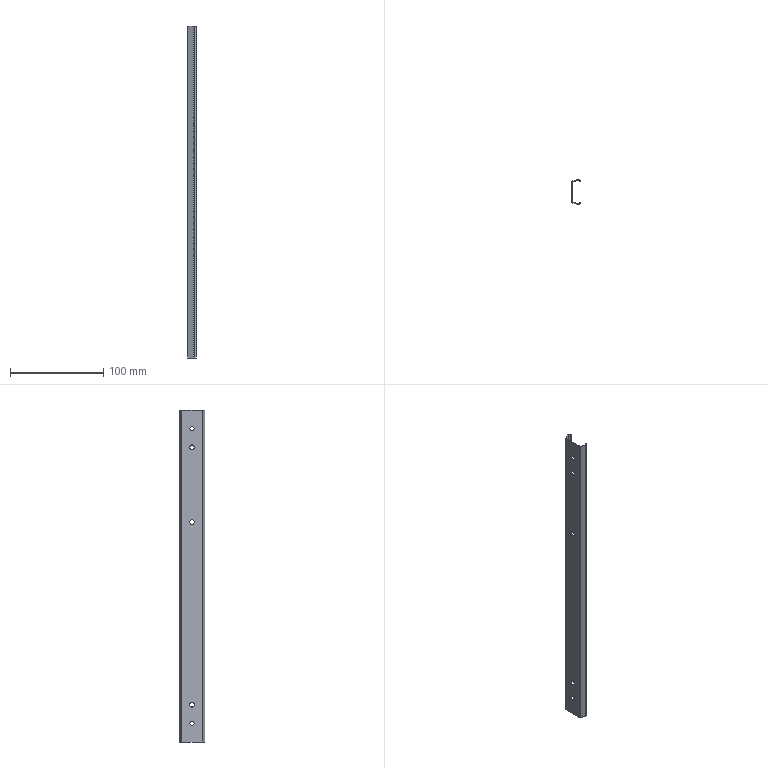Part | SolidWorks | features BaseBody 1, RefAxis 1 | 1 solid | 37 faces | box 9 x 27 x 355.6 mm | volume 7594 mm3 | plane 20 | cylinder 17 | commonest cylinder face diameters 4.5 x13 3.7 x2 3.8 x2
STEP:
#1=CARTESIAN_POINT('',(-2.55,11.15,333.35));
#2=VERTEX_POINT('',#1);
#3=CARTESIAN_POINT('',(-2.55,11.15,337.85));
#4=VERTEX_POINT('',#3);
#5=CARTESIAN_POINT('',(-2.55,11.15,335.6));
#6=DIRECTION('',(-1.,0.,0.));
#7=DIRECTION('',(0.,0.,1.));
#8=AXIS2_PLACEMENT_3D('',#5,#6,#7);
#9=CIRCLE('',#8,2.25);
#10=EDGE_CURVE('',#2,#4,#9,.T.);
#11=ORIENTED_EDGE('',*,*,#10,.F.);
#12=CARTESIAN_POINT('',(-3.05,11.15,333.35));
#13=VERTEX_POINT('',#12);
#14=CARTESIAN_POINT('',(-3.05,11.15,333.35));
#15=DIRECTION('',(-1.,0.,0.));
#16=VECTOR('',#15,1000.);
#17=LINE('',#14,#16);
#18=EDGE_CURVE('',#2,#13,#17,.T.);
#19=ORIENTED_EDGE('',*,*,#18,.T.);
#20=CARTESIAN_POINT('',(-3.05,11.15,337.85));
#21=VERTEX_POINT('',#20);
#22=CARTESIAN_POINT('',(-3.05,11.15,335.6));
#23=DIRECTION('',(1.,0.,0.));
#24=DIRECTION('',(0.,0.,1.));
#25=AXIS2_PLACEMENT_3D('',#22,#23,#24);
#26=CIRCLE('',#25,2.25);
#27=EDGE_CURVE('',#21,#13,#26,.T.);
#28=ORIENTED_EDGE('',*,*,#27,.F.);
#29=CARTESIAN_POINT('',(-3.05,11.15,337.85));
#30=DIRECTION('',(-1.,0.,0.));
#31=VECTOR('',#30,1000.);
#32=LINE('',#29,#31);
#33=EDGE_CURVE('',#4,#21,#32,.T.);
#34=ORIENTED_EDGE('',*,*,#33,.F.);
#35=EDGE_LOOP('',(#11,#19,#28,#34));
#36=FACE_OUTER_BOUND('',#35,.T.);
#37=CARTESIAN_POINT('',(-3.05,11.15,335.6));
#38=DIRECTION('',(-1.,0.,0.));
#39=DIRECTION('',(0.,0.,1.));
#40=AXIS2_PLACEMENT_3D('',#37,#38,#39);
#41=CYLINDRICAL_SURFACE('',#40,2.25);
#42=ADVANCED_FACE('',(#36),#41,.F.);
#43=CARTESIAN_POINT('',(-2.55,11.15,17.75));
#44=VERTEX_POINT('',#43);
#45=CARTESIAN_POINT('',(-2.55,11.15,22.25));
#46=VERTEX_POINT('',#45);
#47=CARTESIAN_POINT('',(-2.55,11.15,20.));
#48=DIRECTION('',(-1.,0.,0.));
#49=DIRECTION('',(0.,0.,1.));
#50=AXIS2_PLACEMENT_3D('',#47,#48,#49);
#51=CIRCLE('',#50,2.25);
#52=EDGE_CURVE('',#44,#46,#51,.T.);
#53=ORIENTED_EDGE('',*,*,#52,.F.);
#54=CARTESIAN_POINT('',(-3.05,11.15,17.75));
#55=VERTEX_POINT('',#54);
#56=CARTESIAN_POINT('',(-3.05,11.15,17.75));
#57=DIRECTION('',(-1.,0.,0.));
#58=VECTOR('',#57,1000.);
#59=LINE('',#56,#58);
#60=EDGE_CURVE('',#44,#55,#59,.T.);
#61=ORIENTED_EDGE('',*,*,#60,.T.);
#62=CARTESIAN_POINT('',(-3.05,11.15,22.25));
#63=VERTEX_POINT('',#62);
#64=CARTESIAN_POINT('',(-3.05,11.15,20.));
#65=DIRECTION('',(1.,0.,0.));
#66=DIRECTION('',(0.,0.,1.));
#67=AXIS2_PLACEMENT_3D('',#64,#65,#66);
#68=CIRCLE('',#67,2.25);
#69=EDGE_CURVE('',#63,#55,#68,.T.);
#70=ORIENTED_EDGE('',*,*,#69,.F.);
#71=CARTESIAN_POINT('',(-3.05,11.15,22.25));
#72=DIRECTION('',(-1.,0.,0.));
#73=VECTOR('',#72,1000.);
#74=LINE('',#71,#73);
#75=EDGE_CURVE('',#46,#63,#74,.T.);
#76=ORIENTED_EDGE('',*,*,#75,.F.);
#77=EDGE_LOOP('',(#53,#61,#70,#76));
#78=FACE_OUTER_BOUND('',#77,.T.);
#79=CARTESIAN_POINT('',(-3.05,11.15,20.));
#80=DIRECTION('',(-1.,0.,0.));
#81=DIRECTION('',(0.,0.,1.));
#82=AXIS2_PLACEMENT_3D('',#79,#80,#81);
#83=CYLINDRICAL_SURFACE('',#82,2.25);
#84=ADVANCED_FACE('',(#78),#83,.F.);
#85=CARTESIAN_POINT('',(-2.55,11.15,318.25));
#86=VERTEX_POINT('',#85);
#87=CARTESIAN_POINT('',(-2.55,13.4,316.));
#88=VERTEX_POINT('',#87);
#89=CARTESIAN_POINT('',(-2.55,11.15,316.));
#90=DIRECTION('',(-1.,0.,0.));
#91=DIRECTION('',(0.,0.,1.));
#92=AXIS2_PLACEMENT_3D('',#89,#90,#91);
#93=CIRCLE('',#92,2.25);
#94=EDGE_CURVE('',#86,#88,#93,.T.);
#95=ORIENTED_EDGE('',*,*,#94,.F.);
#96=CARTESIAN_POINT('',(-3.05,11.15,318.25));
#97=VERTEX_POINT('',#96);
#98=CARTESIAN_POINT('',(-3.05,11.15,318.25));
#99=DIRECTION('',(-1.,0.,0.));
#100=VECTOR('',#99,1000.);
#101=LINE('',#98,#100);
#102=EDGE_CURVE('',#86,#97,#101,.T.);
#103=ORIENTED_EDGE('',*,*,#102,.T.);
#104=CARTESIAN_POINT('',(-3.05,13.4,316.));
#105=VERTEX_POINT('',#104);
#106=CARTESIAN_POINT('',(-3.05,11.15,316.));
#107=DIRECTION('',(1.,0.,0.));
#108=DIRECTION('',(0.,0.,1.));
#109=AXIS2_PLACEMENT_3D('',#106,#107,#108);
#110=CIRCLE('',#109,2.25);
#111=EDGE_CURVE('',#105,#97,#110,.T.);
#112=ORIENTED_EDGE('',*,*,#111,.F.);
#113=CARTESIAN_POINT('',(-3.05,13.4,316.));
#114=DIRECTION('',(1.,0.,0.));
#115=VECTOR('',#114,1000.);
#116=LINE('',#113,#115);
#117=EDGE_CURVE('',#105,#88,#116,.T.);
#118=ORIENTED_EDGE('',*,*,#117,.T.);
#119=EDGE_LOOP('',(#95,#103,#112,#118));
#120=FACE_OUTER_BOUND('',#119,.T.);
#121=CARTESIAN_POINT('',(-3.05,11.15,316.));
#122=DIRECTION('',(-1.,0.,0.));
#123=DIRECTION('',(0.,0.,1.));
#124=AXIS2_PLACEMENT_3D('',#121,#122,#123);
#125=CYLINDRICAL_SURFACE('',#124,2.25);
#126=ADVANCED_FACE('',(#120),#125,.F.);
#127=CARTESIAN_POINT('',(-2.55,11.15,42.65));
#128=VERTEX_POINT('',#127);
#129=CARTESIAN_POINT('',(-2.55,13.4,40.4));
#130=VERTEX_POINT('',#129);
#131=CARTESIAN_POINT('',(-2.55,11.15,40.4));
#132=DIRECTION('',(-1.,0.,0.));
#133=DIRECTION('',(0.,0.,1.));
#134=AXIS2_PLACEMENT_3D('',#131,#132,#133);
#135=CIRCLE('',#134,2.25);
#136=EDGE_CURVE('',#128,#130,#135,.T.);
#137=ORIENTED_EDGE('',*,*,#136,.F.);
#138=CARTESIAN_POINT('',(-3.05,11.15,42.65));
#139=VERTEX_POINT('',#138);
#140=CARTESIAN_POINT('',(-3.05,11.15,42.65));
#141=DIRECTION('',(-1.,0.,0.));
#142=VECTOR('',#141,1000.);
#143=LINE('',#140,#142);
#144=EDGE_CURVE('',#128,#139,#143,.T.);
#145=ORIENTED_EDGE('',*,*,#144,.T.);
#146=CARTESIAN_POINT('',(-3.05,13.4,40.4));
#147=VERTEX_POINT('',#146);
#148=CARTESIAN_POINT('',(-3.05,11.15,40.4));
#149=DIRECTION('',(1.,0.,0.));
#150=DIRECTION('',(0.,0.,1.));
#151=AXIS2_PLACEMENT_3D('',#148,#149,#150);
#152=CIRCLE('',#151,2.25);
#153=EDGE_CURVE('',#147,#139,#152,.T.);
#154=ORIENTED_EDGE('',*,*,#153,.F.);
#155=CARTESIAN_POINT('',(-3.05,13.4,40.4));
#156=DIRECTION('',(1.,0.,0.));
#157=VECTOR('',#156,1000.);
#158=LINE('',#155,#157);
#159=EDGE_CURVE('',#147,#130,#158,.T.);
#160=ORIENTED_EDGE('',*,*,#159,.T.);
#161=EDGE_LOOP('',(#137,#145,#154,#160));
#162=FACE_OUTER_BOUND('',#161,.T.);
#163=CARTESIAN_POINT('',(-3.05,11.15,40.4));
#164=DIRECTION('',(-1.,0.,0.));
#165=DIRECTION('',(0.,0.,1.));
#166=AXIS2_PLACEMENT_3D('',#163,#164,#165);
#167=CYLINDRICAL_SURFACE('',#166,2.25);
#168=ADVANCED_FACE('',(#162),#167,.F.);
#169=CARTESIAN_POINT('',(-2.55,11.15,238.25));
#170=VERTEX_POINT('',#169);
#171=CARTESIAN_POINT('',(-2.55,13.4,236.));
#172=VERTEX_POINT('',#171);
#173=CARTESIAN_POINT('',(-2.55,11.15,236.));
#174=DIRECTION('',(-1.,0.,0.));
#175=DIRECTION('',(0.,0.,1.));
#176=AXIS2_PLACEMENT_3D('',#173,#174,#175);
#177=CIRCLE('',#176,2.25);
#178=EDGE_CURVE('',#170,#172,#177,.T.);
#179=ORIENTED_EDGE('',*,*,#178,.F.);
#180=CARTESIAN_POINT('',(-3.05,11.15,238.25));
#181=VERTEX_POINT('',#180);
#182=CARTESIAN_POINT('',(-3.05,11.15,238.25));
#183=DIRECTION('',(-1.,0.,0.));
#184=VECTOR('',#183,1000.);
#185=LINE('',#182,#184);
#186=EDGE_CURVE('',#170,#181,#185,.T.);
#187=ORIENTED_EDGE('',*,*,#186,.T.);
#188=CARTESIAN_POINT('',(-3.05,13.4,236.));
#189=VERTEX_POINT('',#188);
#190=CARTESIAN_POINT('',(-3.05,11.15,236.));
#191=DIRECTION('',(1.,0.,0.));
#192=DIRECTION('',(0.,0.,1.));
#193=AXIS2_PLACEMENT_3D('',#190,#191,#192);
#194=CIRCLE('',#193,2.25);
#195=EDGE_CURVE('',#189,#181,#194,.T.);
#196=ORIENTED_EDGE('',*,*,#195,.F.);
#197=CARTESIAN_POINT('',(-3.05,13.4,236.));
#198=DIRECTION('',(1.,0.,0.));
#199=VECTOR('',#198,1000.);
#200=LINE('',#197,#199);
#201=EDGE_CURVE('',#189,#172,#200,.T.);
#202=ORIENTED_EDGE('',*,*,#201,.T.);
#203=EDGE_LOOP('',(#179,#187,#196,#202));
#204=FACE_OUTER_BOUND('',#203,.T.);
#205=CARTESIAN_POINT('',(-3.05,11.15,236.));
#206=DIRECTION('',(-1.,0.,0.));
#207=DIRECTION('',(0.,0.,1.));
#208=AXIS2_PLACEMENT_3D('',#205,#206,#207);
#209=CYLINDRICAL_SURFACE('',#208,2.25);
#210=ADVANCED_FACE('',(#204),#209,.F.);
#211=CARTESIAN_POINT('',(-3.05,22.248,0.));
#212=VERTEX_POINT('',#211);
#213=CARTESIAN_POINT('',(-3.05,0.05184,0.));
#214=VERTEX_POINT('',#213);
#215=CARTESIAN_POINT('',(-3.05,0.05184,0.));
#216=DIRECTION('',(0.,-1.,0.));
#217=VECTOR('',#216,1000.);
#218=LINE('',#215,#217);
#219=EDGE_CURVE('',#212,#214,#218,.T.);
#220=ORIENTED_EDGE('',*,*,#219,.T.);
#221=CARTESIAN_POINT('',(-3.05,0.05184,355.6));
#222=VERTEX_POINT('',#221);
#223=CARTESIAN_POINT('',(-3.05,0.05184,0.));
#224=DIRECTION('',(0.,0.,1.));
#225=VECTOR('',#224,1000.);
#226=LINE('',#223,#225);
#227=EDGE_CURVE('',#214,#222,#226,.T.);
#228=ORIENTED_EDGE('',*,*,#227,.T.);
#229=CARTESIAN_POINT('',(-3.05,22.248,355.6));
#230=VERTEX_POINT('',#229);
#231=CARTESIAN_POINT('',(-3.05,0.05184,355.6));
#232=DIRECTION('',(0.,1.,0.));
#233=VECTOR('',#232,1000.);
#234=LINE('',#231,#233);
#235=EDGE_CURVE('',#222,#230,#234,.T.);
#236=ORIENTED_EDGE('',*,*,#235,.T.);
#237=CARTESIAN_POINT('',(-3.05,22.248,0.));
#238=DIRECTION('',(0.,0.,-1.));
#239=VECTOR('',#238,1000.);
#240=LINE('',#237,#239);
#241=EDGE_CURVE('',#230,#212,#240,.T.);
#242=ORIENTED_EDGE('',*,*,#241,.T.);
#243=EDGE_LOOP('',(#220,#228,#236,#242));
#244=FACE_OUTER_BOUND('',#243,.T.);
#245=ORIENTED_EDGE('',*,*,#27,.T.);
#246=CARTESIAN_POINT('',(-3.05,11.15,335.6));
#247=DIRECTION('',(1.,0.,0.));
#248=DIRECTION('',(0.,0.,1.));
#249=AXIS2_PLACEMENT_3D('',#246,#247,#248);
#250=CIRCLE('',#249,2.25);
#251=EDGE_CURVE('',#13,#21,#250,.T.);
#252=ORIENTED_EDGE('',*,*,#251,.T.);
#253=EDGE_LOOP('',(#245,#252));
#254=FACE_BOUND('',#253,.T.);
#255=ORIENTED_EDGE('',*,*,#69,.T.);
#256=CARTESIAN_POINT('',(-3.05,11.15,20.));
#257=DIRECTION('',(1.,0.,0.));
#258=DIRECTION('',(0.,0.,1.));
#259=AXIS2_PLACEMENT_3D('',#256,#257,#258);
#260=CIRCLE('',#259,2.25);
#261=EDGE_CURVE('',#55,#63,#260,.T.);
#262=ORIENTED_EDGE('',*,*,#261,.T.);
#263=EDGE_LOOP('',(#255,#262));
#264=FACE_BOUND('',#263,.T.);
#265=CARTESIAN_POINT('',(-3.05,8.9,315.2));
#266=VERTEX_POINT('',#265);
#267=CARTESIAN_POINT('',(-3.05,13.4,315.2));
#268=VERTEX_POINT('',#267);
#269=CARTESIAN_POINT('',(-3.05,11.15,315.2));
#270=DIRECTION('',(1.,0.,0.));
#271=DIRECTION('',(0.,0.,1.));
#272=AXIS2_PLACEMENT_3D('',#269,#270,#271);
#273=CIRCLE('',#272,2.25);
#274=EDGE_CURVE('',#266,#268,#273,.T.);
#275=ORIENTED_EDGE('',*,*,#274,.T.);
#276=CARTESIAN_POINT('',(-3.05,13.4,0.));
#277=DIRECTION('',(0.,0.,1.));
#278=VECTOR('',#277,1000.);
#279=LINE('',#276,#278);
#280=EDGE_CURVE('',#268,#105,#279,.T.);
#281=ORIENTED_EDGE('',*,*,#280,.T.);
#282=ORIENTED_EDGE('',*,*,#111,.T.);
#283=CARTESIAN_POINT('',(-3.05,8.9,316.));
#284=VERTEX_POINT('',#283);
#285=CARTESIAN_POINT('',(-3.05,11.15,316.));
#286=DIRECTION('',(1.,0.,0.));
#287=DIRECTION('',(0.,0.,1.));
#288=AXIS2_PLACEMENT_3D('',#285,#286,#287);
#289=CIRCLE('',#288,2.25);
#290=EDGE_CURVE('',#97,#284,#289,.T.);
#291=ORIENTED_EDGE('',*,*,#290,.T.);
#292=CARTESIAN_POINT('',(-3.05,8.9,0.));
#293=DIRECTION('',(0.,0.,-1.));
#294=VECTOR('',#293,1000.);
#295=LINE('',#292,#294);
#296=EDGE_CURVE('',#284,#266,#295,.T.);
#297=ORIENTED_EDGE('',*,*,#296,.T.);
#298=EDGE_LOOP('',(#275,#281,#282,#291,#297));
#299=FACE_BOUND('',#298,.T.);
#300=CARTESIAN_POINT('',(-3.05,8.9,39.6));
#301=VERTEX_POINT('',#300);
#302=CARTESIAN_POINT('',(-3.05,13.4,39.6));
#303=VERTEX_POINT('',#302);
#304=CARTESIAN_POINT('',(-3.05,11.15,39.6));
#305=DIRECTION('',(1.,0.,0.));
#306=DIRECTION('',(0.,0.,1.));
#307=AXIS2_PLACEMENT_3D('',#304,#305,#306);
#308=CIRCLE('',#307,2.25);
#309=EDGE_CURVE('',#301,#303,#308,.T.);
#310=ORIENTED_EDGE('',*,*,#309,.T.);
#311=CARTESIAN_POINT('',(-3.05,13.4,0.));
#312=DIRECTION('',(0.,0.,1.));
#313=VECTOR('',#312,1000.);
#314=LINE('',#311,#313);
#315=EDGE_CURVE('',#303,#147,#314,.T.);
#316=ORIENTED_EDGE('',*,*,#315,.T.);
#317=ORIENTED_EDGE('',*,*,#153,.T.);
#318=CARTESIAN_POINT('',(-3.05,8.9,40.4));
#319=VERTEX_POINT('',#318);
#320=CARTESIAN_POINT('',(-3.05,11.15,40.4));
#321=DIRECTION('',(1.,0.,0.));
#322=DIRECTION('',(0.,0.,1.));
#323=AXIS2_PLACEMENT_3D('',#320,#321,#322);
#324=CIRCLE('',#323,2.25);
#325=EDGE_CURVE('',#139,#319,#324,.T.);
#326=ORIENTED_EDGE('',*,*,#325,.T.);
#327=CARTESIAN_POINT('',(-3.05,8.9,0.));
#328=DIRECTION('',(0.,0.,-1.));
#329=VECTOR('',#328,1000.);
#330=LINE('',#327,#329);
#331=EDGE_CURVE('',#319,#301,#330,.T.);
#332=ORIENTED_EDGE('',*,*,#331,.T.);
#333=EDGE_LOOP('',(#310,#316,#317,#326,#332));
#334=FACE_BOUND('',#333,.T.);
#335=CARTESIAN_POINT('',(-3.05,8.9,235.2));
#336=VERTEX_POINT('',#335);
#337=CARTESIAN_POINT('',(-3.05,13.4,235.2));
#338=VERTEX_POINT('',#337);
#339=CARTESIAN_POINT('',(-3.05,11.15,235.2));
#340=DIRECTION('',(1.,0.,0.));
#341=DIRECTION('',(0.,0.,1.));
#342=AXIS2_PLACEMENT_3D('',#339,#340,#341);
#343=CIRCLE('',#342,2.25);
#344=EDGE_CURVE('',#336,#338,#343,.T.);
#345=ORIENTED_EDGE('',*,*,#344,.T.);
#346=CARTESIAN_POINT('',(-3.05,13.4,0.));
#347=DIRECTION('',(0.,0.,1.));
#348=VECTOR('',#347,1000.);
#349=LINE('',#346,#348);
#350=EDGE_CURVE('',#338,#189,#349,.T.);
#351=ORIENTED_EDGE('',*,*,#350,.T.);
#352=ORIENTED_EDGE('',*,*,#195,.T.);
#353=CARTESIAN_POINT('',(-3.05,8.9,236.));
#354=VERTEX_POINT('',#353);
#355=CARTESIAN_POINT('',(-3.05,11.15,236.));
#356=DIRECTION('',(1.,0.,0.));
#357=DIRECTION('',(0.,0.,1.));
#358=AXIS2_PLACEMENT_3D('',#355,#356,#357);
#359=CIRCLE('',#358,2.25);
#360=EDGE_CURVE('',#181,#354,#359,.T.);
#361=ORIENTED_EDGE('',*,*,#360,.T.);
#362=CARTESIAN_POINT('',(-3.05,8.9,0.));
#363=DIRECTION('',(0.,0.,-1.));
#364=VECTOR('',#363,1000.);
#365=LINE('',#362,#364);
#366=EDGE_CURVE('',#354,#336,#365,.T.);
#367=ORIENTED_EDGE('',*,*,#366,.T.);
#368=EDGE_LOOP('',(#345,#351,#352,#361,#367));
#369=FACE_BOUND('',#368,.T.);
#370=CARTESIAN_POINT('',(-3.05,0.05184,0.));
#371=DIRECTION('',(-1.,0.,0.));
#372=DIRECTION('',(0.,0.,1.));
#373=AXIS2_PLACEMENT_3D('',#370,#371,#372);
#374=PLANE('',#373);
#375=ADVANCED_FACE('',(#244,#254,#264,#299,#334,#369),#374,.T.);
#376=CARTESIAN_POINT('',(3.016,-2.35,0.));
#377=VERTEX_POINT('',#376);
#378=CARTESIAN_POINT('',(3.016,-2.35,0.));
#379=DIRECTION('',(0.9298,-0.3681,0.));
#380=VECTOR('',#379,1000.);
#381=LINE('',#378,#380);
#382=EDGE_CURVE('',#214,#377,#381,.T.);
#383=ORIENTED_EDGE('',*,*,#382,.T.);
#384=CARTESIAN_POINT('',(3.016,-2.35,355.6));
#385=VERTEX_POINT('',#384);
#386=CARTESIAN_POINT('',(3.016,-2.35,0.));
#387=DIRECTION('',(0.,0.,1.));
#388=VECTOR('',#387,1000.);
#389=LINE('',#386,#388);
#390=EDGE_CURVE('',#377,#385,#389,.T.);
#391=ORIENTED_EDGE('',*,*,#390,.T.);
#392=CARTESIAN_POINT('',(3.016,-2.35,355.6));
#393=DIRECTION('',(-0.9298,0.3681,0.));
#394=VECTOR('',#393,1000.);
#395=LINE('',#392,#394);
#396=EDGE_CURVE('',#385,#222,#395,.T.);
#397=ORIENTED_EDGE('',*,*,#396,.T.);
#398=ORIENTED_EDGE('',*,*,#227,.F.);
#399=EDGE_LOOP('',(#383,#391,#397,#398));
#400=FACE_OUTER_BOUND('',#399,.T.);
#401=CARTESIAN_POINT('',(3.016,-2.35,0.));
#402=DIRECTION('',(-0.3681,-0.9298,0.));
#403=DIRECTION('',(0.9298,-0.3681,0.));
#404=AXIS2_PLACEMENT_3D('',#401,#402,#403);
#405=PLANE('',#404);
#406=ADVANCED_FACE('',(#400),#405,.T.);
#407=CARTESIAN_POINT('',(3.016,24.65,0.));
#408=VERTEX_POINT('',#407);
#409=CARTESIAN_POINT('',(3.016,24.65,0.));
#410=DIRECTION('',(-0.9298,-0.3681,0.));
#411=VECTOR('',#410,1000.);
#412=LINE('',#409,#411);
#413=EDGE_CURVE('',#408,#212,#412,.T.);
#414=ORIENTED_EDGE('',*,*,#413,.F.);
#415=CARTESIAN_POINT('',(4.1,24.65,0.));
#416=VERTEX_POINT('',#415);
#417=CARTESIAN_POINT('',(3.016,24.65,0.));
#418=DIRECTION('',(-1.,0.,0.));
#419=VECTOR('',#418,1000.);
#420=LINE('',#417,#419);
#421=EDGE_CURVE('',#416,#408,#420,.T.);
#422=ORIENTED_EDGE('',*,*,#421,.F.);
#423=CARTESIAN_POINT('',(5.95,22.8,0.));
#424=VERTEX_POINT('',#423);
#425=CARTESIAN_POINT('',(4.1,22.8,0.));
#426=DIRECTION('',(0.,0.,1.));
#427=DIRECTION('',(-1.,0.,0.));
#428=AXIS2_PLACEMENT_3D('',#425,#426,#427);
#429=CIRCLE('',#428,1.85);
#430=EDGE_CURVE('',#424,#416,#429,.T.);
#431=ORIENTED_EDGE('',*,*,#430,.F.);
#432=CARTESIAN_POINT('',(5.95,22.506,0.));
#433=VERTEX_POINT('',#432);
#434=CARTESIAN_POINT('',(5.95,22.8,0.));
#435=DIRECTION('',(0.,1.,0.));
#436=VECTOR('',#435,1000.);
#437=LINE('',#434,#436);
#438=EDGE_CURVE('',#433,#424,#437,.T.);
#439=ORIENTED_EDGE('',*,*,#438,.F.);
#440=CARTESIAN_POINT('',(5.493,22.466,0.));
#441=VERTEX_POINT('',#440);
#442=CARTESIAN_POINT('',(5.95,22.506,0.));
#443=DIRECTION('',(0.9962,0.08716,0.));
#444=VECTOR('',#443,1000.);
#445=LINE('',#442,#444);
#446=EDGE_CURVE('',#441,#433,#445,.T.);
#447=ORIENTED_EDGE('',*,*,#446,.F.);
#448=CARTESIAN_POINT('',(2.901,24.067,0.));
#449=VERTEX_POINT('',#448);
#450=CARTESIAN_POINT('',(3.6,22.3,0.));
#451=DIRECTION('',(0.,0.,-1.));
#452=DIRECTION('',(-1.,0.,0.));
#453=AXIS2_PLACEMENT_3D('',#450,#451,#452);
#454=CIRCLE('',#453,1.9);
#455=EDGE_CURVE('',#449,#441,#454,.T.);
#456=ORIENTED_EDGE('',*,*,#455,.F.);
#457=CARTESIAN_POINT('',(-2.55,21.908,0.));
#458=VERTEX_POINT('',#457);
#459=CARTESIAN_POINT('',(-2.55,21.908,0.));
#460=DIRECTION('',(0.9298,0.3681,0.));
#461=VECTOR('',#460,1000.);
#462=LINE('',#459,#461);
#463=EDGE_CURVE('',#458,#449,#462,.T.);
#464=ORIENTED_EDGE('',*,*,#463,.F.);
#465=CARTESIAN_POINT('',(-2.55,0.3916,0.));
#466=VERTEX_POINT('',#465);
#467=CARTESIAN_POINT('',(-2.55,-2.35,0.));
#468=DIRECTION('',(0.,1.,0.));
#469=VECTOR('',#468,1000.);
#470=LINE('',#467,#469);
#471=EDGE_CURVE('',#466,#458,#470,.T.);
#472=ORIENTED_EDGE('',*,*,#471,.F.);
#473=CARTESIAN_POINT('',(2.901,-1.767,0.));
#474=VERTEX_POINT('',#473);
#475=CARTESIAN_POINT('',(2.901,-1.767,0.));
#476=DIRECTION('',(-0.9298,0.3681,0.));
#477=VECTOR('',#476,1000.);
#478=LINE('',#475,#477);
#479=EDGE_CURVE('',#474,#466,#478,.T.);
#480=ORIENTED_EDGE('',*,*,#479,.F.);
#481=CARTESIAN_POINT('',(5.493,-0.1656,0.));
#482=VERTEX_POINT('',#481);
#483=CARTESIAN_POINT('',(3.6,0.,0.));
#484=DIRECTION('',(0.,0.,-1.));
#485=DIRECTION('',(-1.,0.,0.));
#486=AXIS2_PLACEMENT_3D('',#483,#484,#485);
#487=CIRCLE('',#486,1.9);
#488=EDGE_CURVE('',#482,#474,#487,.T.);
#489=ORIENTED_EDGE('',*,*,#488,.F.);
#490=CARTESIAN_POINT('',(5.95,-0.2056,0.));
#491=VERTEX_POINT('',#490);
#492=CARTESIAN_POINT('',(5.493,-0.1656,0.));
#493=DIRECTION('',(-0.9962,0.08716,0.));
#494=VECTOR('',#493,1000.);
#495=LINE('',#492,#494);
#496=EDGE_CURVE('',#491,#482,#495,.T.);
#497=ORIENTED_EDGE('',*,*,#496,.F.);
#498=CARTESIAN_POINT('',(5.95,-0.5,0.));
#499=VERTEX_POINT('',#498);
#500=CARTESIAN_POINT('',(5.95,-0.2056,0.));
#501=DIRECTION('',(0.,1.,0.));
#502=VECTOR('',#501,1000.);
#503=LINE('',#500,#502);
#504=EDGE_CURVE('',#499,#491,#503,.T.);
#505=ORIENTED_EDGE('',*,*,#504,.F.);
#506=CARTESIAN_POINT('',(4.1,-2.35,0.));
#507=VERTEX_POINT('',#506);
#508=CARTESIAN_POINT('',(4.1,-0.5,0.));
#509=DIRECTION('',(0.,0.,1.));
#510=DIRECTION('',(-1.,0.,0.));
#511=AXIS2_PLACEMENT_3D('',#508,#509,#510);
#512=CIRCLE('',#511,1.85);
#513=EDGE_CURVE('',#507,#499,#512,.T.);
#514=ORIENTED_EDGE('',*,*,#513,.F.);
#515=CARTESIAN_POINT('',(-3.05,-2.35,0.));
#516=DIRECTION('',(1.,0.,0.));
#517=VECTOR('',#516,1000.);
#518=LINE('',#515,#517);
#519=EDGE_CURVE('',#377,#507,#518,.T.);
#520=ORIENTED_EDGE('',*,*,#519,.F.);
#521=ORIENTED_EDGE('',*,*,#382,.F.);
#522=ORIENTED_EDGE('',*,*,#219,.F.);
#523=EDGE_LOOP('',(#414,#422,#431,#439,#447,#456,#464,#472,#480,#489,#497,#505,#514,#520,#521,#522));
#524=FACE_OUTER_BOUND('',#523,.T.);
#525=CARTESIAN_POINT('',(-3.05,-2.35,0.));
#526=DIRECTION('',(0.,0.,1.));
#527=DIRECTION('',(1.,0.,0.));
#528=AXIS2_PLACEMENT_3D('',#525,#526,#527);
#529=PLANE('',#528);
#530=ADVANCED_FACE('',(#524),#529,.F.);
#531=ORIENTED_EDGE('',*,*,#413,.T.);
#532=ORIENTED_EDGE('',*,*,#241,.F.);
#533=CARTESIAN_POINT('',(3.016,24.65,355.6));
#534=VERTEX_POINT('',#533);
#535=CARTESIAN_POINT('',(-3.05,22.248,355.6));
#536=DIRECTION('',(0.9298,0.3681,0.));
#537=VECTOR('',#536,1000.);
#538=LINE('',#535,#537);
#539=EDGE_CURVE('',#230,#534,#538,.T.);
#540=ORIENTED_EDGE('',*,*,#539,.T.);
#541=CARTESIAN_POINT('',(3.016,24.65,0.));
#542=DIRECTION('',(0.,0.,-1.));
#543=VECTOR('',#542,1000.);
#544=LINE('',#541,#543);
#545=EDGE_CURVE('',#534,#408,#544,.T.);
#546=ORIENTED_EDGE('',*,*,#545,.T.);
#547=EDGE_LOOP('',(#531,#532,#540,#546));
#548=FACE_OUTER_BOUND('',#547,.T.);
#549=CARTESIAN_POINT('',(-3.05,22.248,0.));
#550=DIRECTION('',(-0.3681,0.9298,0.));
#551=DIRECTION('',(-0.9298,-0.3681,0.));
#552=AXIS2_PLACEMENT_3D('',#549,#550,#551);
#553=PLANE('',#552);
#554=ADVANCED_FACE('',(#548),#553,.T.);
#555=CARTESIAN_POINT('',(5.95,22.8,355.6));
#556=VERTEX_POINT('',#555);
#557=CARTESIAN_POINT('',(4.1,24.65,355.6));
#558=VERTEX_POINT('',#557);
#559=CARTESIAN_POINT('',(4.1,22.8,355.6));
#560=DIRECTION('',(0.,0.,1.));
#561=DIRECTION('',(-1.,0.,0.));
#562=AXIS2_PLACEMENT_3D('',#559,#560,#561);
#563=CIRCLE('',#562,1.85);
#564=EDGE_CURVE('',#556,#558,#563,.T.);
#565=ORIENTED_EDGE('',*,*,#564,.T.);
#566=CARTESIAN_POINT('',(-3.05,24.65,355.6));
#567=DIRECTION('',(-1.,0.,0.));
#568=VECTOR('',#567,1000.);
#569=LINE('',#566,#568);
#570=EDGE_CURVE('',#558,#534,#569,.T.);
#571=ORIENTED_EDGE('',*,*,#570,.T.);
#572=ORIENTED_EDGE('',*,*,#539,.F.);
#573=ORIENTED_EDGE('',*,*,#235,.F.);
#574=ORIENTED_EDGE('',*,*,#396,.F.);
#575=CARTESIAN_POINT('',(4.1,-2.35,355.6));
#576=VERTEX_POINT('',#575);
#577=CARTESIAN_POINT('',(-3.05,-2.35,355.6));
#578=DIRECTION('',(1.,0.,0.));
#579=VECTOR('',#578,1000.);
#580=LINE('',#577,#579);
#581=EDGE_CURVE('',#385,#576,#580,.T.);
#582=ORIENTED_EDGE('',*,*,#581,.T.);
#583=CARTESIAN_POINT('',(5.95,-0.5,355.6));
#584=VERTEX_POINT('',#583);
#585=CARTESIAN_POINT('',(4.1,-0.5,355.6));
#586=DIRECTION('',(0.,0.,1.));
#587=DIRECTION('',(-1.,0.,0.));
#588=AXIS2_PLACEMENT_3D('',#585,#586,#587);
#589=CIRCLE('',#588,1.85);
#590=EDGE_CURVE('',#576,#584,#589,.T.);
#591=ORIENTED_EDGE('',*,*,#590,.T.);
#592=CARTESIAN_POINT('',(5.95,-0.2056,355.6));
#593=VERTEX_POINT('',#592);
#594=CARTESIAN_POINT('',(5.95,-0.2056,355.6));
#595=DIRECTION('',(0.,-1.,0.));
#596=VECTOR('',#595,1000.);
#597=LINE('',#594,#596);
#598=EDGE_CURVE('',#593,#584,#597,.T.);
#599=ORIENTED_EDGE('',*,*,#598,.F.);
#600=CARTESIAN_POINT('',(5.493,-0.1656,355.6));
#601=VERTEX_POINT('',#600);
#602=CARTESIAN_POINT('',(5.493,-0.1656,355.6));
#603=DIRECTION('',(0.9962,-0.08716,0.));
#604=VECTOR('',#603,1000.);
#605=LINE('',#602,#604);
#606=EDGE_CURVE('',#601,#593,#605,.T.);
#607=ORIENTED_EDGE('',*,*,#606,.F.);
#608=CARTESIAN_POINT('',(2.901,-1.767,355.6));
#609=VERTEX_POINT('',#608);
#610=CARTESIAN_POINT('',(3.6,0.,355.6));
#611=DIRECTION('',(0.,0.,-1.));
#612=DIRECTION('',(-1.,0.,0.));
#613=AXIS2_PLACEMENT_3D('',#610,#611,#612);
#614=CIRCLE('',#613,1.9);
#615=EDGE_CURVE('',#601,#609,#614,.T.);
#616=ORIENTED_EDGE('',*,*,#615,.T.);
#617=CARTESIAN_POINT('',(-2.55,0.3916,355.6));
#618=VERTEX_POINT('',#617);
#619=CARTESIAN_POINT('',(2.901,-1.767,355.6));
#620=DIRECTION('',(-0.9298,0.3681,0.));
#621=VECTOR('',#620,1000.);
#622=LINE('',#619,#621);
#623=EDGE_CURVE('',#609,#618,#622,.T.);
#624=ORIENTED_EDGE('',*,*,#623,.T.);
#625=CARTESIAN_POINT('',(-2.55,21.908,355.6));
#626=VERTEX_POINT('',#625);
#627=CARTESIAN_POINT('',(-2.55,-2.35,355.6));
#628=DIRECTION('',(0.,1.,0.));
#629=VECTOR('',#628,1000.);
#630=LINE('',#627,#629);
#631=EDGE_CURVE('',#618,#626,#630,.T.);
#632=ORIENTED_EDGE('',*,*,#631,.T.);
#633=CARTESIAN_POINT('',(2.901,24.067,355.6));
#634=VERTEX_POINT('',#633);
#635=CARTESIAN_POINT('',(-2.55,21.908,355.6));
#636=DIRECTION('',(0.9298,0.3681,0.));
#637=VECTOR('',#636,1000.);
#638=LINE('',#635,#637);
#639=EDGE_CURVE('',#626,#634,#638,.T.);
#640=ORIENTED_EDGE('',*,*,#639,.T.);
#641=CARTESIAN_POINT('',(5.493,22.466,355.6));
#642=VERTEX_POINT('',#641);
#643=CARTESIAN_POINT('',(3.6,22.3,355.6));
#644=DIRECTION('',(0.,0.,-1.));
#645=DIRECTION('',(-1.,0.,0.));
#646=AXIS2_PLACEMENT_3D('',#643,#644,#645);
#647=CIRCLE('',#646,1.9);
#648=EDGE_CURVE('',#634,#642,#647,.T.);
#649=ORIENTED_EDGE('',*,*,#648,.T.);
#650=CARTESIAN_POINT('',(5.95,22.506,355.6));
#651=VERTEX_POINT('',#650);
#652=CARTESIAN_POINT('',(5.95,22.506,355.6));
#653=DIRECTION('',(-0.9962,-0.08716,0.));
#654=VECTOR('',#653,1000.);
#655=LINE('',#652,#654);
#656=EDGE_CURVE('',#651,#642,#655,.T.);
#657=ORIENTED_EDGE('',*,*,#656,.F.);
#658=CARTESIAN_POINT('',(5.95,22.8,355.6));
#659=DIRECTION('',(0.,-1.,0.));
#660=VECTOR('',#659,1000.);
#661=LINE('',#658,#660);
#662=EDGE_CURVE('',#556,#651,#661,.T.);
#663=ORIENTED_EDGE('',*,*,#662,.F.);
#664=EDGE_LOOP('',(#565,#571,#572,#573,#574,#582,#591,#599,#607,#616,#624,#632,#640,#649,#657,#663));
#665=FACE_OUTER_BOUND('',#664,.T.);
#666=CARTESIAN_POINT('',(-3.05,-2.35,355.6));
#667=DIRECTION('',(0.,0.,1.));
#668=DIRECTION('',(1.,0.,0.));
#669=AXIS2_PLACEMENT_3D('',#666,#667,#668);
#670=PLANE('',#669);
#671=ADVANCED_FACE('',(#665),#670,.T.);
#672=ORIENTED_EDGE('',*,*,#18,.F.);
#673=CARTESIAN_POINT('',(-2.55,11.15,335.6));
#674=DIRECTION('',(-1.,0.,0.));
#675=DIRECTION('',(0.,0.,1.));
#676=AXIS2_PLACEMENT_3D('',#673,#674,#675);
#677=CIRCLE('',#676,2.25);
#678=EDGE_CURVE('',#4,#2,#677,.T.);
#679=ORIENTED_EDGE('',*,*,#678,.F.);
#680=ORIENTED_EDGE('',*,*,#33,.T.);
#681=ORIENTED_EDGE('',*,*,#251,.F.);
#682=EDGE_LOOP('',(#672,#679,#680,#681));
#683=FACE_OUTER_BOUND('',#682,.T.);
#684=CARTESIAN_POINT('',(-3.05,11.15,335.6));
#685=DIRECTION('',(-1.,0.,0.));
#686=DIRECTION('',(0.,0.,1.));
#687=AXIS2_PLACEMENT_3D('',#684,#685,#686);
#688=CYLINDRICAL_SURFACE('',#687,2.25);
#689=ADVANCED_FACE('',(#683),#688,.F.);
#690=ORIENTED_EDGE('',*,*,#60,.F.);
#691=CARTESIAN_POINT('',(-2.55,11.15,20.));
#692=DIRECTION('',(-1.,0.,0.));
#693=DIRECTION('',(0.,0.,1.));
#694=AXIS2_PLACEMENT_3D('',#691,#692,#693);
#695=CIRCLE('',#694,2.25);
#696=EDGE_CURVE('',#46,#44,#695,.T.);
#697=ORIENTED_EDGE('',*,*,#696,.F.);
#698=ORIENTED_EDGE('',*,*,#75,.T.);
#699=ORIENTED_EDGE('',*,*,#261,.F.);
#700=EDGE_LOOP('',(#690,#697,#698,#699));
#701=FACE_OUTER_BOUND('',#700,.T.);
#702=CARTESIAN_POINT('',(-3.05,11.15,20.));
#703=DIRECTION('',(-1.,0.,0.));
#704=DIRECTION('',(0.,0.,1.));
#705=AXIS2_PLACEMENT_3D('',#702,#703,#704);
#706=CYLINDRICAL_SURFACE('',#705,2.25);
#707=ADVANCED_FACE('',(#701),#706,.F.);
#708=ORIENTED_EDGE('',*,*,#117,.F.);
#709=ORIENTED_EDGE('',*,*,#280,.F.);
#710=CARTESIAN_POINT('',(-2.55,13.4,315.2));
#711=VERTEX_POINT('',#710);
#712=CARTESIAN_POINT('',(-3.05,13.4,315.2));
#713=DIRECTION('',(-1.,0.,0.));
#714=VECTOR('',#713,1000.);
#715=LINE('',#712,#714);
#716=EDGE_CURVE('',#711,#268,#715,.T.);
#717=ORIENTED_EDGE('',*,*,#716,.F.);
#718=CARTESIAN_POINT('',(-2.55,13.4,316.));
#719=DIRECTION('',(0.,0.,-1.));
#720=VECTOR('',#719,1000.);
#721=LINE('',#718,#720);
#722=EDGE_CURVE('',#88,#711,#721,.T.);
#723=ORIENTED_EDGE('',*,*,#722,.F.);
#724=EDGE_LOOP('',(#708,#709,#717,#723));
#725=FACE_OUTER_BOUND('',#724,.T.);
#726=CARTESIAN_POINT('',(-3.05,13.4,316.));
#727=DIRECTION('',(0.,1.,0.));
#728=DIRECTION('',(0.,0.,1.));
#729=AXIS2_PLACEMENT_3D('',#726,#727,#728);
#730=PLANE('',#729);
#731=ADVANCED_FACE('',(#725),#730,.F.);
#732=ORIENTED_EDGE('',*,*,#716,.T.);
#733=ORIENTED_EDGE('',*,*,#274,.F.);
#734=CARTESIAN_POINT('',(-2.55,8.9,315.2));
#735=VERTEX_POINT('',#734);
#736=CARTESIAN_POINT('',(-3.05,8.9,315.2));
#737=DIRECTION('',(-1.,0.,0.));
#738=VECTOR('',#737,1000.);
#739=LINE('',#736,#738);
#740=EDGE_CURVE('',#735,#266,#739,.T.);
#741=ORIENTED_EDGE('',*,*,#740,.F.);
#742=CARTESIAN_POINT('',(-2.55,11.15,315.2));
#743=DIRECTION('',(-1.,0.,0.));
#744=DIRECTION('',(0.,0.,1.));
#745=AXIS2_PLACEMENT_3D('',#742,#743,#744);
#746=CIRCLE('',#745,2.25);
#747=EDGE_CURVE('',#711,#735,#746,.T.);
#748=ORIENTED_EDGE('',*,*,#747,.F.);
#749=EDGE_LOOP('',(#732,#733,#741,#748));
#750=FACE_OUTER_BOUND('',#749,.T.);
#751=CARTESIAN_POINT('',(-3.05,11.15,315.2));
#752=DIRECTION('',(-1.,0.,0.));
#753=DIRECTION('',(0.,0.,1.));
#754=AXIS2_PLACEMENT_3D('',#751,#752,#753);
#755=CYLINDRICAL_SURFACE('',#754,2.25);
#756=ADVANCED_FACE('',(#750),#755,.F.);
#757=ORIENTED_EDGE('',*,*,#740,.T.);
#758=ORIENTED_EDGE('',*,*,#296,.F.);
#759=CARTESIAN_POINT('',(-2.55,8.9,316.));
#760=VERTEX_POINT('',#759);
#761=CARTESIAN_POINT('',(-3.05,8.9,316.));
#762=DIRECTION('',(-1.,0.,0.));
#763=VECTOR('',#762,1000.);
#764=LINE('',#761,#763);
#765=EDGE_CURVE('',#760,#284,#764,.T.);
#766=ORIENTED_EDGE('',*,*,#765,.F.);
#767=CARTESIAN_POINT('',(-2.55,8.9,315.2));
#768=DIRECTION('',(0.,0.,1.));
#769=VECTOR('',#768,1000.);
#770=LINE('',#767,#769);
#771=EDGE_CURVE('',#735,#760,#770,.T.);
#772=ORIENTED_EDGE('',*,*,#771,.F.);
#773=EDGE_LOOP('',(#757,#758,#766,#772));
#774=FACE_OUTER_BOUND('',#773,.T.);
#775=CARTESIAN_POINT('',(-3.05,8.9,315.2));
#776=DIRECTION('',(0.,-1.,0.));
#777=DIRECTION('',(0.,0.,-1.));
#778=AXIS2_PLACEMENT_3D('',#775,#776,#777);
#779=PLANE('',#778);
#780=ADVANCED_FACE('',(#774),#779,.F.);
#781=ORIENTED_EDGE('',*,*,#102,.F.);
#782=CARTESIAN_POINT('',(-2.55,11.15,316.));
#783=DIRECTION('',(-1.,0.,0.));
#784=DIRECTION('',(0.,0.,1.));
#785=AXIS2_PLACEMENT_3D('',#782,#783,#784);
#786=CIRCLE('',#785,2.25);
#787=EDGE_CURVE('',#760,#86,#786,.T.);
#788=ORIENTED_EDGE('',*,*,#787,.F.);
#789=ORIENTED_EDGE('',*,*,#765,.T.);
#790=ORIENTED_EDGE('',*,*,#290,.F.);
#791=EDGE_LOOP('',(#781,#788,#789,#790));
#792=FACE_OUTER_BOUND('',#791,.T.);
#793=CARTESIAN_POINT('',(-3.05,11.15,316.));
#794=DIRECTION('',(-1.,0.,0.));
#795=DIRECTION('',(0.,0.,1.));
#796=AXIS2_PLACEMENT_3D('',#793,#794,#795);
#797=CYLINDRICAL_SURFACE('',#796,2.25);
#798=ADVANCED_FACE('',(#792),#797,.F.);
#799=ORIENTED_EDGE('',*,*,#159,.F.);
#800=ORIENTED_EDGE('',*,*,#315,.F.);
#801=CARTESIAN_POINT('',(-2.55,13.4,39.6));
#802=VERTEX_POINT('',#801);
#803=CARTESIAN_POINT('',(-3.05,13.4,39.6));
#804=DIRECTION('',(-1.,0.,0.));
#805=VECTOR('',#804,1000.);
#806=LINE('',#803,#805);
#807=EDGE_CURVE('',#802,#303,#806,.T.);
#808=ORIENTED_EDGE('',*,*,#807,.F.);
#809=CARTESIAN_POINT('',(-2.55,13.4,40.4));
#810=DIRECTION('',(0.,0.,-1.));
#811=VECTOR('',#810,1000.);
#812=LINE('',#809,#811);
#813=EDGE_CURVE('',#130,#802,#812,.T.);
#814=ORIENTED_EDGE('',*,*,#813,.F.);
#815=EDGE_LOOP('',(#799,#800,#808,#814));
#816=FACE_OUTER_BOUND('',#815,.T.);
#817=CARTESIAN_POINT('',(-3.05,13.4,40.4));
#818=DIRECTION('',(0.,1.,0.));
#819=DIRECTION('',(0.,0.,1.));
#820=AXIS2_PLACEMENT_3D('',#817,#818,#819);
#821=PLANE('',#820);
#822=ADVANCED_FACE('',(#816),#821,.F.);
#823=ORIENTED_EDGE('',*,*,#807,.T.);
#824=ORIENTED_EDGE('',*,*,#309,.F.);
#825=CARTESIAN_POINT('',(-2.55,8.9,39.6));
#826=VERTEX_POINT('',#825);
#827=CARTESIAN_POINT('',(-3.05,8.9,39.6));
#828=DIRECTION('',(-1.,0.,0.));
#829=VECTOR('',#828,1000.);
#830=LINE('',#827,#829);
#831=EDGE_CURVE('',#826,#301,#830,.T.);
#832=ORIENTED_EDGE('',*,*,#831,.F.);
#833=CARTESIAN_POINT('',(-2.55,11.15,39.6));
#834=DIRECTION('',(-1.,0.,0.));
#835=DIRECTION('',(0.,0.,1.));
#836=AXIS2_PLACEMENT_3D('',#833,#834,#835);
#837=CIRCLE('',#836,2.25);
#838=EDGE_CURVE('',#802,#826,#837,.T.);
#839=ORIENTED_EDGE('',*,*,#838,.F.);
#840=EDGE_LOOP('',(#823,#824,#832,#839));
#841=FACE_OUTER_BOUND('',#840,.T.);
#842=CARTESIAN_POINT('',(-3.05,11.15,39.6));
#843=DIRECTION('',(-1.,0.,0.));
#844=DIRECTION('',(0.,0.,1.));
#845=AXIS2_PLACEMENT_3D('',#842,#843,#844);
#846=CYLINDRICAL_SURFACE('',#845,2.25);
#847=ADVANCED_FACE('',(#841),#846,.F.);
#848=ORIENTED_EDGE('',*,*,#831,.T.);
#849=ORIENTED_EDGE('',*,*,#331,.F.);
#850=CARTESIAN_POINT('',(-2.55,8.9,40.4));
#851=VERTEX_POINT('',#850);
#852=CARTESIAN_POINT('',(-3.05,8.9,40.4));
#853=DIRECTION('',(-1.,0.,0.));
#854=VECTOR('',#853,1000.);
#855=LINE('',#852,#854);
#856=EDGE_CURVE('',#851,#319,#855,.T.);
#857=ORIENTED_EDGE('',*,*,#856,.F.);
#858=CARTESIAN_POINT('',(-2.55,8.9,39.6));
#859=DIRECTION('',(0.,0.,1.));
#860=VECTOR('',#859,1000.);
#861=LINE('',#858,#860);
#862=EDGE_CURVE('',#826,#851,#861,.T.);
#863=ORIENTED_EDGE('',*,*,#862,.F.);
#864=EDGE_LOOP('',(#848,#849,#857,#863));
#865=FACE_OUTER_BOUND('',#864,.T.);
#866=CARTESIAN_POINT('',(-3.05,8.9,39.6));
#867=DIRECTION('',(0.,-1.,0.));
#868=DIRECTION('',(0.,0.,-1.));
#869=AXIS2_PLACEMENT_3D('',#866,#867,#868);
#870=PLANE('',#869);
#871=ADVANCED_FACE('',(#865),#870,.F.);
#872=ORIENTED_EDGE('',*,*,#144,.F.);
#873=CARTESIAN_POINT('',(-2.55,11.15,40.4));
#874=DIRECTION('',(-1.,0.,0.));
#875=DIRECTION('',(0.,0.,1.));
#876=AXIS2_PLACEMENT_3D('',#873,#874,#875);
#877=CIRCLE('',#876,2.25);
#878=EDGE_CURVE('',#851,#128,#877,.T.);
#879=ORIENTED_EDGE('',*,*,#878,.F.);
#880=ORIENTED_EDGE('',*,*,#856,.T.);
#881=ORIENTED_EDGE('',*,*,#325,.F.);
#882=EDGE_LOOP('',(#872,#879,#880,#881));
#883=FACE_OUTER_BOUND('',#882,.T.);
#884=CARTESIAN_POINT('',(-3.05,11.15,40.4));
#885=DIRECTION('',(-1.,0.,0.));
#886=DIRECTION('',(0.,0.,1.));
#887=AXIS2_PLACEMENT_3D('',#884,#885,#886);
#888=CYLINDRICAL_SURFACE('',#887,2.25);
#889=ADVANCED_FACE('',(#883),#888,.F.);
#890=ORIENTED_EDGE('',*,*,#201,.F.);
#891=ORIENTED_EDGE('',*,*,#350,.F.);
#892=CARTESIAN_POINT('',(-2.55,13.4,235.2));
#893=VERTEX_POINT('',#892);
#894=CARTESIAN_POINT('',(-3.05,13.4,235.2));
#895=DIRECTION('',(-1.,0.,0.));
#896=VECTOR('',#895,1000.);
#897=LINE('',#894,#896);
#898=EDGE_CURVE('',#893,#338,#897,.T.);
#899=ORIENTED_EDGE('',*,*,#898,.F.);
#900=CARTESIAN_POINT('',(-2.55,13.4,236.));
#901=DIRECTION('',(0.,0.,-1.));
#902=VECTOR('',#901,1000.);
#903=LINE('',#900,#902);
#904=EDGE_CURVE('',#172,#893,#903,.T.);
#905=ORIENTED_EDGE('',*,*,#904,.F.);
#906=EDGE_LOOP('',(#890,#891,#899,#905));
#907=FACE_OUTER_BOUND('',#906,.T.);
#908=CARTESIAN_POINT('',(-3.05,13.4,236.));
#909=DIRECTION('',(0.,1.,0.));
#910=DIRECTION('',(0.,0.,1.));
#911=AXIS2_PLACEMENT_3D('',#908,#909,#910);
#912=PLANE('',#911);
#913=ADVANCED_FACE('',(#907),#912,.F.);
#914=ORIENTED_EDGE('',*,*,#898,.T.);
#915=ORIENTED_EDGE('',*,*,#344,.F.);
#916=CARTESIAN_POINT('',(-2.55,8.9,235.2));
#917=VERTEX_POINT('',#916);
#918=CARTESIAN_POINT('',(-3.05,8.9,235.2));
#919=DIRECTION('',(-1.,0.,0.));
#920=VECTOR('',#919,1000.);
#921=LINE('',#918,#920);
#922=EDGE_CURVE('',#917,#336,#921,.T.);
#923=ORIENTED_EDGE('',*,*,#922,.F.);
#924=CARTESIAN_POINT('',(-2.55,11.15,235.2));
#925=DIRECTION('',(-1.,0.,0.));
#926=DIRECTION('',(0.,0.,1.));
#927=AXIS2_PLACEMENT_3D('',#924,#925,#926);
#928=CIRCLE('',#927,2.25);
#929=EDGE_CURVE('',#893,#917,#928,.T.);
#930=ORIENTED_EDGE('',*,*,#929,.F.);
#931=EDGE_LOOP('',(#914,#915,#923,#930));
#932=FACE_OUTER_BOUND('',#931,.T.);
#933=CARTESIAN_POINT('',(-3.05,11.15,235.2));
#934=DIRECTION('',(-1.,0.,0.));
#935=DIRECTION('',(0.,0.,1.));
#936=AXIS2_PLACEMENT_3D('',#933,#934,#935);
#937=CYLINDRICAL_SURFACE('',#936,2.25);
#938=ADVANCED_FACE('',(#932),#937,.F.);
#939=ORIENTED_EDGE('',*,*,#922,.T.);
#940=ORIENTED_EDGE('',*,*,#366,.F.);
#941=CARTESIAN_POINT('',(-2.55,8.9,236.));
#942=VERTEX_POINT('',#941);
#943=CARTESIAN_POINT('',(-3.05,8.9,236.));
#944=DIRECTION('',(-1.,0.,0.));
#945=VECTOR('',#944,1000.);
#946=LINE('',#943,#945);
#947=EDGE_CURVE('',#942,#354,#946,.T.);
#948=ORIENTED_EDGE('',*,*,#947,.F.);
#949=CARTESIAN_POINT('',(-2.55,8.9,235.2));
#950=DIRECTION('',(0.,0.,1.));
#951=VECTOR('',#950,1000.);
#952=LINE('',#949,#951);
#953=EDGE_CURVE('',#917,#942,#952,.T.);
#954=ORIENTED_EDGE('',*,*,#953,.F.);
#955=EDGE_LOOP('',(#939,#940,#948,#954));
#956=FACE_OUTER_BOUND('',#955,.T.);
#957=CARTESIAN_POINT('',(-3.05,8.9,235.2));
#958=DIRECTION('',(0.,-1.,0.));
#959=DIRECTION('',(0.,0.,-1.));
#960=AXIS2_PLACEMENT_3D('',#957,#958,#959);
#961=PLANE('',#960);
#962=ADVANCED_FACE('',(#956),#961,.F.);
#963=ORIENTED_EDGE('',*,*,#186,.F.);
#964=CARTESIAN_POINT('',(-2.55,11.15,236.));
#965=DIRECTION('',(-1.,0.,0.));
#966=DIRECTION('',(0.,0.,1.));
#967=AXIS2_PLACEMENT_3D('',#964,#965,#966);
#968=CIRCLE('',#967,2.25);
#969=EDGE_CURVE('',#942,#170,#968,.T.);
#970=ORIENTED_EDGE('',*,*,#969,.F.);
#971=ORIENTED_EDGE('',*,*,#947,.T.);
#972=ORIENTED_EDGE('',*,*,#360,.F.);
#973=EDGE_LOOP('',(#963,#970,#971,#972));
#974=FACE_OUTER_BOUND('',#973,.T.);
#975=CARTESIAN_POINT('',(-3.05,11.15,236.));
#976=DIRECTION('',(-1.,0.,0.));
#977=DIRECTION('',(0.,0.,1.));
#978=AXIS2_PLACEMENT_3D('',#975,#976,#977);
#979=CYLINDRICAL_SURFACE('',#978,2.25);
#980=ADVANCED_FACE('',(#974),#979,.F.);
#981=ORIENTED_EDGE('',*,*,#519,.T.);
#982=CARTESIAN_POINT('',(4.1,-2.35,0.));
#983=DIRECTION('',(0.,0.,1.));
#984=VECTOR('',#983,1000.);
#985=LINE('',#982,#984);
#986=EDGE_CURVE('',#507,#576,#985,.T.);
#987=ORIENTED_EDGE('',*,*,#986,.T.);
#988=ORIENTED_EDGE('',*,*,#581,.F.);
#989=ORIENTED_EDGE('',*,*,#390,.F.);
#990=EDGE_LOOP('',(#981,#987,#988,#989));
#991=FACE_OUTER_BOUND('',#990,.T.);
#992=CARTESIAN_POINT('',(4.1,-2.35,0.));
#993=DIRECTION('',(0.,-1.,0.));
#994=DIRECTION('',(0.,0.,-1.));
#995=AXIS2_PLACEMENT_3D('',#992,#993,#994);
#996=PLANE('',#995);
#997=ADVANCED_FACE('',(#991),#996,.T.);
#998=ORIENTED_EDGE('',*,*,#430,.T.);
#999=CARTESIAN_POINT('',(4.1,24.65,0.));
#1000=DIRECTION('',(0.,0.,1.));
#1001=VECTOR('',#1000,1000.);
#1002=LINE('',#999,#1001);
#1003=EDGE_CURVE('',#416,#558,#1002,.T.);
#1004=ORIENTED_EDGE('',*,*,#1003,.T.);
#1005=ORIENTED_EDGE('',*,*,#564,.F.);
#1006=CARTESIAN_POINT('',(5.95,22.8,0.));
#1007=DIRECTION('',(0.,0.,-1.));
#1008=VECTOR('',#1007,1000.);
#1009=LINE('',#1006,#1008);
#1010=EDGE_CURVE('',#556,#424,#1009,.T.);
#1011=ORIENTED_EDGE('',*,*,#1010,.T.);
#1012=EDGE_LOOP('',(#998,#1004,#1005,#1011));
#1013=FACE_OUTER_BOUND('',#1012,.T.);
#1014=CARTESIAN_POINT('',(4.1,22.8,0.));
#1015=DIRECTION('',(0.,0.,-1.));
#1016=DIRECTION('',(-1.,0.,0.));
#1017=AXIS2_PLACEMENT_3D('',#1014,#1015,#1016);
#1018=CYLINDRICAL_SURFACE('',#1017,1.85);
#1019=ADVANCED_FACE('',(#1013),#1018,.T.);
#1020=CARTESIAN_POINT('',(2.901,24.067,0.));
#1021=DIRECTION('',(0.,0.,1.));
#1022=VECTOR('',#1021,1000.);
#1023=LINE('',#1020,#1022);
#1024=EDGE_CURVE('',#449,#634,#1023,.T.);
#1025=ORIENTED_EDGE('',*,*,#1024,.F.);
#1026=ORIENTED_EDGE('',*,*,#455,.T.);
#1027=CARTESIAN_POINT('',(5.493,22.466,0.));
#1028=DIRECTION('',(0.,0.,-1.));
#1029=VECTOR('',#1028,1000.);
#1030=LINE('',#1027,#1029);
#1031=EDGE_CURVE('',#642,#441,#1030,.T.);
#1032=ORIENTED_EDGE('',*,*,#1031,.F.);
#1033=ORIENTED_EDGE('',*,*,#648,.F.);
#1034=EDGE_LOOP('',(#1025,#1026,#1032,#1033));
#1035=FACE_OUTER_BOUND('',#1034,.T.);
#1036=CARTESIAN_POINT('',(3.6,22.3,0.));
#1037=DIRECTION('',(0.,0.,-1.));
#1038=DIRECTION('',(-1.,0.,0.));
#1039=AXIS2_PLACEMENT_3D('',#1036,#1037,#1038);
#1040=CYLINDRICAL_SURFACE('',#1039,1.9);
#1041=ADVANCED_FACE('',(#1035),#1040,.F.);
#1042=ORIENTED_EDGE('',*,*,#463,.T.);
#1043=ORIENTED_EDGE('',*,*,#1024,.T.);
#1044=ORIENTED_EDGE('',*,*,#639,.F.);
#1045=CARTESIAN_POINT('',(-2.55,21.908,0.));
#1046=DIRECTION('',(0.,0.,-1.));
#1047=VECTOR('',#1046,1000.);
#1048=LINE('',#1045,#1047);
#1049=EDGE_CURVE('',#626,#458,#1048,.T.);
#1050=ORIENTED_EDGE('',*,*,#1049,.T.);
#1051=EDGE_LOOP('',(#1042,#1043,#1044,#1050));
#1052=FACE_OUTER_BOUND('',#1051,.T.);
#1053=CARTESIAN_POINT('',(2.901,24.067,0.));
#1054=DIRECTION('',(0.3681,-0.9298,0.));
#1055=DIRECTION('',(0.9298,0.3681,0.));
#1056=AXIS2_PLACEMENT_3D('',#1053,#1054,#1055);
#1057=PLANE('',#1056);
#1058=ADVANCED_FACE('',(#1052),#1057,.T.);
#1059=ORIENTED_EDGE('',*,*,#471,.T.);
#1060=ORIENTED_EDGE('',*,*,#1049,.F.);
#1061=ORIENTED_EDGE('',*,*,#631,.F.);
#1062=CARTESIAN_POINT('',(-2.55,0.3916,0.));
#1063=DIRECTION('',(0.,0.,-1.));
#1064=VECTOR('',#1063,1000.);
#1065=LINE('',#1062,#1064);
#1066=EDGE_CURVE('',#618,#466,#1065,.T.);
#1067=ORIENTED_EDGE('',*,*,#1066,.T.);
#1068=EDGE_LOOP('',(#1059,#1060,#1061,#1067));
#1069=FACE_OUTER_BOUND('',#1068,.T.);
#1070=ORIENTED_EDGE('',*,*,#678,.T.);
#1071=ORIENTED_EDGE('',*,*,#10,.T.);
#1072=EDGE_LOOP('',(#1070,#1071));
#1073=FACE_BOUND('',#1072,.T.);
#1074=ORIENTED_EDGE('',*,*,#696,.T.);
#1075=ORIENTED_EDGE('',*,*,#52,.T.);
#1076=EDGE_LOOP('',(#1074,#1075));
#1077=FACE_BOUND('',#1076,.T.);
#1078=ORIENTED_EDGE('',*,*,#747,.T.);
#1079=ORIENTED_EDGE('',*,*,#771,.T.);
#1080=ORIENTED_EDGE('',*,*,#787,.T.);
#1081=ORIENTED_EDGE('',*,*,#94,.T.);
#1082=ORIENTED_EDGE('',*,*,#722,.T.);
#1083=EDGE_LOOP('',(#1078,#1079,#1080,#1081,#1082));
#1084=FACE_BOUND('',#1083,.T.);
#1085=ORIENTED_EDGE('',*,*,#838,.T.);
#1086=ORIENTED_EDGE('',*,*,#862,.T.);
#1087=ORIENTED_EDGE('',*,*,#878,.T.);
#1088=ORIENTED_EDGE('',*,*,#136,.T.);
#1089=ORIENTED_EDGE('',*,*,#813,.T.);
#1090=EDGE_LOOP('',(#1085,#1086,#1087,#1088,#1089));
#1091=FACE_BOUND('',#1090,.T.);
#1092=ORIENTED_EDGE('',*,*,#929,.T.);
#1093=ORIENTED_EDGE('',*,*,#953,.T.);
#1094=ORIENTED_EDGE('',*,*,#969,.T.);
#1095=ORIENTED_EDGE('',*,*,#178,.T.);
#1096=ORIENTED_EDGE('',*,*,#904,.T.);
#1097=EDGE_LOOP('',(#1092,#1093,#1094,#1095,#1096));
#1098=FACE_BOUND('',#1097,.T.);
#1099=CARTESIAN_POINT('',(-2.55,21.908,0.));
#1100=DIRECTION('',(1.,0.,0.));
#1101=DIRECTION('',(0.,0.,-1.));
#1102=AXIS2_PLACEMENT_3D('',#1099,#1100,#1101);
#1103=PLANE('',#1102);
#1104=ADVANCED_FACE('',(#1069,#1073,#1077,#1084,#1091,#1098),#1103,.T.);
#1105=ORIENTED_EDGE('',*,*,#479,.T.);
#1106=ORIENTED_EDGE('',*,*,#1066,.F.);
#1107=ORIENTED_EDGE('',*,*,#623,.F.);
#1108=CARTESIAN_POINT('',(2.901,-1.767,0.));
#1109=DIRECTION('',(0.,0.,-1.));
#1110=VECTOR('',#1109,1000.);
#1111=LINE('',#1108,#1110);
#1112=EDGE_CURVE('',#609,#474,#1111,.T.);
#1113=ORIENTED_EDGE('',*,*,#1112,.T.);
#1114=EDGE_LOOP('',(#1105,#1106,#1107,#1113));
#1115=FACE_OUTER_BOUND('',#1114,.T.);
#1116=CARTESIAN_POINT('',(-2.55,0.3916,0.));
#1117=DIRECTION('',(0.3681,0.9298,0.));
#1118=DIRECTION('',(-0.9298,0.3681,0.));
#1119=AXIS2_PLACEMENT_3D('',#1116,#1117,#1118);
#1120=PLANE('',#1119);
#1121=ADVANCED_FACE('',(#1115),#1120,.T.);
#1122=CARTESIAN_POINT('',(5.493,-0.1656,0.));
#1123=DIRECTION('',(0.,0.,1.));
#1124=VECTOR('',#1123,1000.);
#1125=LINE('',#1122,#1124);
#1126=EDGE_CURVE('',#482,#601,#1125,.T.);
#1127=ORIENTED_EDGE('',*,*,#1126,.F.);
#1128=ORIENTED_EDGE('',*,*,#488,.T.);
#1129=ORIENTED_EDGE('',*,*,#1112,.F.);
#1130=ORIENTED_EDGE('',*,*,#615,.F.);
#1131=EDGE_LOOP('',(#1127,#1128,#1129,#1130));
#1132=FACE_OUTER_BOUND('',#1131,.T.);
#1133=CARTESIAN_POINT('',(3.6,0.,0.));
#1134=DIRECTION('',(0.,0.,-1.));
#1135=DIRECTION('',(-1.,0.,0.));
#1136=AXIS2_PLACEMENT_3D('',#1133,#1134,#1135);
#1137=CYLINDRICAL_SURFACE('',#1136,1.9);
#1138=ADVANCED_FACE('',(#1132),#1137,.F.);
#1139=ORIENTED_EDGE('',*,*,#513,.T.);
#1140=CARTESIAN_POINT('',(5.95,-0.5,0.));
#1141=DIRECTION('',(0.,0.,1.));
#1142=VECTOR('',#1141,1000.);
#1143=LINE('',#1140,#1142);
#1144=EDGE_CURVE('',#499,#584,#1143,.T.);
#1145=ORIENTED_EDGE('',*,*,#1144,.T.);
#1146=ORIENTED_EDGE('',*,*,#590,.F.);
#1147=ORIENTED_EDGE('',*,*,#986,.F.);
#1148=EDGE_LOOP('',(#1139,#1145,#1146,#1147));
#1149=FACE_OUTER_BOUND('',#1148,.T.);
#1150=CARTESIAN_POINT('',(4.1,-0.5,0.));
#1151=DIRECTION('',(0.,0.,-1.));
#1152=DIRECTION('',(-1.,0.,0.));
#1153=AXIS2_PLACEMENT_3D('',#1150,#1151,#1152);
#1154=CYLINDRICAL_SURFACE('',#1153,1.85);
#1155=ADVANCED_FACE('',(#1149),#1154,.T.);
#1156=ORIENTED_EDGE('',*,*,#421,.T.);
#1157=ORIENTED_EDGE('',*,*,#545,.F.);
#1158=ORIENTED_EDGE('',*,*,#570,.F.);
#1159=ORIENTED_EDGE('',*,*,#1003,.F.);
#1160=EDGE_LOOP('',(#1156,#1157,#1158,#1159));
#1161=FACE_OUTER_BOUND('',#1160,.T.);
#1162=CARTESIAN_POINT('',(3.016,24.65,0.));
#1163=DIRECTION('',(0.,1.,0.));
#1164=DIRECTION('',(0.,0.,1.));
#1165=AXIS2_PLACEMENT_3D('',#1162,#1163,#1164);
#1166=PLANE('',#1165);
#1167=ADVANCED_FACE('',(#1161),#1166,.T.);
#1168=ORIENTED_EDGE('',*,*,#438,.T.);
#1169=ORIENTED_EDGE('',*,*,#1010,.F.);
#1170=ORIENTED_EDGE('',*,*,#662,.T.);
#1171=CARTESIAN_POINT('',(5.95,22.506,0.));
#1172=DIRECTION('',(0.,0.,-1.));
#1173=VECTOR('',#1172,1000.);
#1174=LINE('',#1171,#1173);
#1175=EDGE_CURVE('',#651,#433,#1174,.T.);
#1176=ORIENTED_EDGE('',*,*,#1175,.T.);
#1177=EDGE_LOOP('',(#1168,#1169,#1170,#1176));
#1178=FACE_OUTER_BOUND('',#1177,.T.);
#1179=CARTESIAN_POINT('',(5.95,22.8,0.));
#1180=DIRECTION('',(1.,0.,0.));
#1181=DIRECTION('',(0.,0.,-1.));
#1182=AXIS2_PLACEMENT_3D('',#1179,#1180,#1181);
#1183=PLANE('',#1182);
#1184=ADVANCED_FACE('',(#1178),#1183,.T.);
#1185=ORIENTED_EDGE('',*,*,#446,.T.);
#1186=ORIENTED_EDGE('',*,*,#1175,.F.);
#1187=ORIENTED_EDGE('',*,*,#656,.T.);
#1188=ORIENTED_EDGE('',*,*,#1031,.T.);
#1189=EDGE_LOOP('',(#1185,#1186,#1187,#1188));
#1190=FACE_OUTER_BOUND('',#1189,.T.);
#1191=CARTESIAN_POINT('',(5.95,22.506,0.));
#1192=DIRECTION('',(0.08716,-0.9962,0.));
#1193=DIRECTION('',(0.9962,0.08716,0.));
#1194=AXIS2_PLACEMENT_3D('',#1191,#1192,#1193);
#1195=PLANE('',#1194);
#1196=ADVANCED_FACE('',(#1190),#1195,.T.);
#1197=ORIENTED_EDGE('',*,*,#496,.T.);
#1198=ORIENTED_EDGE('',*,*,#1126,.T.);
#1199=ORIENTED_EDGE('',*,*,#606,.T.);
#1200=CARTESIAN_POINT('',(5.95,-0.2056,0.));
#1201=DIRECTION('',(0.,0.,-1.));
#1202=VECTOR('',#1201,1000.);
#1203=LINE('',#1200,#1202);
#1204=EDGE_CURVE('',#593,#491,#1203,.T.);
#1205=ORIENTED_EDGE('',*,*,#1204,.T.);
#1206=EDGE_LOOP('',(#1197,#1198,#1199,#1205));
#1207=FACE_OUTER_BOUND('',#1206,.T.);
#1208=CARTESIAN_POINT('',(5.493,-0.1656,0.));
#1209=DIRECTION('',(0.08716,0.9962,0.));
#1210=DIRECTION('',(-0.9962,0.08716,0.));
#1211=AXIS2_PLACEMENT_3D('',#1208,#1209,#1210);
#1212=PLANE('',#1211);
#1213=ADVANCED_FACE('',(#1207),#1212,.T.);
#1214=ORIENTED_EDGE('',*,*,#504,.T.);
#1215=ORIENTED_EDGE('',*,*,#1204,.F.);
#1216=ORIENTED_EDGE('',*,*,#598,.T.);
#1217=ORIENTED_EDGE('',*,*,#1144,.F.);
#1218=EDGE_LOOP('',(#1214,#1215,#1216,#1217));
#1219=FACE_OUTER_BOUND('',#1218,.T.);
#1220=CARTESIAN_POINT('',(5.95,-0.2056,0.));
#1221=DIRECTION('',(1.,0.,0.));
#1222=DIRECTION('',(0.,0.,-1.));
#1223=AXIS2_PLACEMENT_3D('',#1220,#1221,#1222);
#1224=PLANE('',#1223);
#1225=ADVANCED_FACE('',(#1219),#1224,.T.);
#1226=CLOSED_SHELL('',(#42,#84,#126,#168,#210,#375,#406,#530,#554,#671,#689,#707,#731,#756,#780,#798,#822,#847,#871,#889,#913,#938,#962,#980,#997,#1019,#1041,#1058,#1104,#1121,#1138,#1155,#1167,#1184,#1196,#1213,#1225));
#1227=MANIFOLD_SOLID_BREP('',#1226);
#1228=CARTESIAN_POINT('',(0.,0.,0.));
#1229=DIRECTION('',(0.,0.,1.));
#1230=DIRECTION('',(1.,0.,0.));
#1231=AXIS2_PLACEMENT_3D('',#1228,#1229,#1230);
#1232=(LENGTH_UNIT()NAMED_UNIT(*)SI_UNIT(.MILLI.,.METRE.));
#1233=UNCERTAINTY_MEASURE_WITH_UNIT(LENGTH_MEASURE(0.00001),#1232,'','');
#1234=(NAMED_UNIT(*)PLANE_ANGLE_UNIT()SI_UNIT($,.RADIAN.));
#1235=(NAMED_UNIT(*)SI_UNIT($,.STERADIAN.)SOLID_ANGLE_UNIT());
#1236=(GEOMETRIC_REPRESENTATION_CONTEXT(3)GLOBAL_UNCERTAINTY_ASSIGNED_CONTEXT((#1233))GLOBAL_UNIT_ASSIGNED_CONTEXT((#1232,#1234,#1235))REPRESENTATION_CONTEXT('',''));
#1237=ADVANCED_BREP_SHAPE_REPRESENTATION('',(#1227,#1231),#1236);